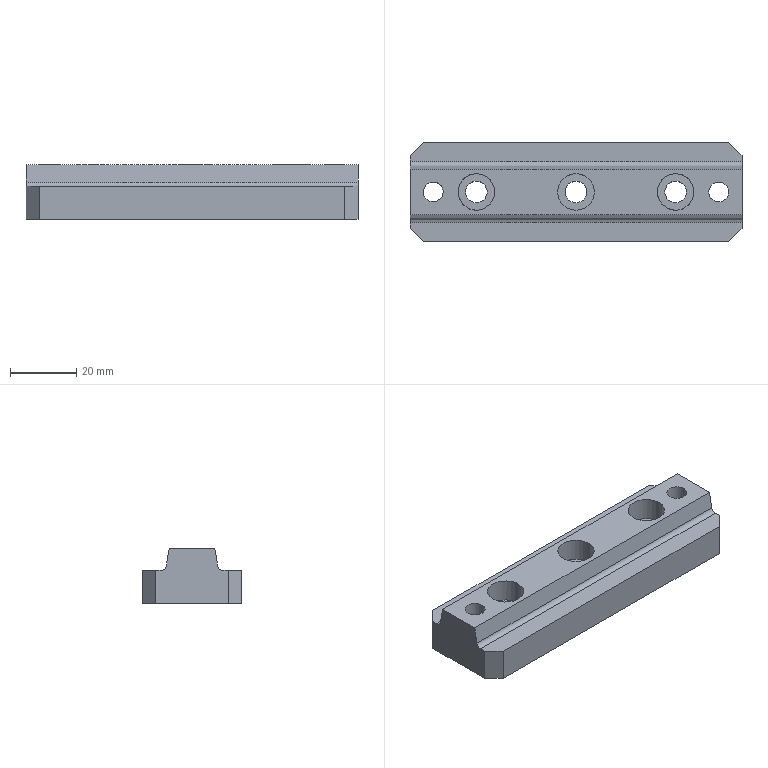Part | STEP file | 车灯-后视镜_id54_x_t | 1 solid | 27 faces | box 100 x 30 x 16.5 mm | volume 35524 mm3 | plane 17 | cylinder 10 | commonest cylinder face diameters 6.5 x3 11 x3 3 x2 6 x2
STEP:
#1=CARTESIAN_POINT('',(46.,250.,-1.5));
#2=VERTEX_POINT('',#1);
#3=CARTESIAN_POINT('',(-46.,250.,-1.5));
#4=VERTEX_POINT('',#3);
#5=CARTESIAN_POINT('',(0.,250.,-1.5));
#6=DIRECTION('',(-1.,0.,0.));
#7=VECTOR('',#6,1.);
#8=LINE('',#5,#7);
#9=EDGE_CURVE('',#2,#4,#8,.T.);
#10=ORIENTED_EDGE('',*,*,#9,.T.);
#11=CARTESIAN_POINT('',(-50.,246.,-1.5));
#12=VERTEX_POINT('',#11);
#13=CARTESIAN_POINT('',(10.75,306.75,-1.5));
#14=DIRECTION('',(0.7071,0.7071,0.));
#15=VECTOR('',#14,1.);
#16=LINE('',#13,#15);
#17=EDGE_CURVE('',#12,#4,#16,.T.);
#18=ORIENTED_EDGE('',*,*,#17,.F.);
#19=CARTESIAN_POINT('',(-50.,244.259,-1.5));
#20=VERTEX_POINT('',#19);
#21=CARTESIAN_POINT('',(-50.,317.5,-1.5));
#22=DIRECTION('',(0.,-1.,0.));
#23=VECTOR('',#22,1.);
#24=LINE('',#21,#23);
#25=EDGE_CURVE('',#12,#20,#24,.T.);
#26=ORIENTED_EDGE('',*,*,#25,.T.);
#27=CARTESIAN_POINT('',(50.,244.259,-1.5));
#28=VERTEX_POINT('',#27);
#29=CARTESIAN_POINT('',(-24.,244.259,-1.5));
#30=DIRECTION('',(-1.,0.,0.));
#31=VECTOR('',#30,1.);
#32=LINE('',#29,#31);
#33=EDGE_CURVE('',#28,#20,#32,.T.);
#34=ORIENTED_EDGE('',*,*,#33,.F.);
#35=CARTESIAN_POINT('',(50.,246.,-1.5));
#36=VERTEX_POINT('',#35);
#37=CARTESIAN_POINT('',(50.,317.5,-1.5));
#38=DIRECTION('',(0.,-1.,0.));
#39=VECTOR('',#38,1.);
#40=LINE('',#37,#39);
#41=EDGE_CURVE('',#36,#28,#40,.T.);
#42=ORIENTED_EDGE('',*,*,#41,.F.);
#43=CARTESIAN_POINT('',(-10.75,306.75,-1.5));
#44=DIRECTION('',(0.7071,-0.7071,0.));
#45=VECTOR('',#44,1.);
#46=LINE('',#43,#45);
#47=EDGE_CURVE('',#2,#36,#46,.T.);
#48=ORIENTED_EDGE('',*,*,#47,.F.);
#49=EDGE_LOOP('',(#10,#18,#26,#34,#42,#48));
#50=FACE_OUTER_BOUND('',#49,.T.);
#51=CARTESIAN_POINT('',(0.,317.5,-1.5));
#52=DIRECTION('',(0.,0.,1.));
#53=DIRECTION('',(1.,0.,0.));
#54=AXIS2_PLACEMENT_3D('',#51,#52,#53);
#55=PLANE('',#54);
#56=ADVANCED_FACE('',(#50),#55,.T.);
#57=CARTESIAN_POINT('',(50.,225.741,-1.5));
#58=VERTEX_POINT('',#57);
#59=CARTESIAN_POINT('',(50.,224.,-1.5));
#60=VERTEX_POINT('',#59);
#61=CARTESIAN_POINT('',(50.,317.5,-1.5));
#62=DIRECTION('',(0.,-1.,0.));
#63=VECTOR('',#62,1.);
#64=LINE('',#61,#63);
#65=EDGE_CURVE('',#58,#60,#64,.T.);
#66=ORIENTED_EDGE('',*,*,#65,.F.);
#67=CARTESIAN_POINT('',(-50.,225.741,-1.5));
#68=VERTEX_POINT('',#67);
#69=CARTESIAN_POINT('',(0.,225.741,-1.5));
#70=DIRECTION('',(1.,0.,0.));
#71=VECTOR('',#70,1.);
#72=LINE('',#69,#71);
#73=EDGE_CURVE('',#68,#58,#72,.T.);
#74=ORIENTED_EDGE('',*,*,#73,.F.);
#75=CARTESIAN_POINT('',(-50.,224.,-1.5));
#76=VERTEX_POINT('',#75);
#77=CARTESIAN_POINT('',(-50.,317.5,-1.5));
#78=DIRECTION('',(0.,-1.,0.));
#79=VECTOR('',#78,1.);
#80=LINE('',#77,#79);
#81=EDGE_CURVE('',#68,#76,#80,.T.);
#82=ORIENTED_EDGE('',*,*,#81,.T.);
#83=CARTESIAN_POINT('',(-46.,220.,-1.5));
#84=VERTEX_POINT('',#83);
#85=CARTESIAN_POINT('',(-71.75,245.75,-1.5));
#86=DIRECTION('',(-0.7071,0.7071,0.));
#87=VECTOR('',#86,1.);
#88=LINE('',#85,#87);
#89=EDGE_CURVE('',#84,#76,#88,.T.);
#90=ORIENTED_EDGE('',*,*,#89,.F.);
#91=CARTESIAN_POINT('',(46.,220.,-1.5));
#92=VERTEX_POINT('',#91);
#93=CARTESIAN_POINT('',(0.,220.,-1.5));
#94=DIRECTION('',(-1.,0.,0.));
#95=VECTOR('',#94,1.);
#96=LINE('',#93,#95);
#97=EDGE_CURVE('',#92,#84,#96,.T.);
#98=ORIENTED_EDGE('',*,*,#97,.F.);
#99=CARTESIAN_POINT('',(71.75,245.75,-1.5));
#100=DIRECTION('',(-0.7071,-0.7071,0.));
#101=VECTOR('',#100,1.);
#102=LINE('',#99,#101);
#103=EDGE_CURVE('',#60,#92,#102,.T.);
#104=ORIENTED_EDGE('',*,*,#103,.F.);
#105=EDGE_LOOP('',(#66,#74,#82,#90,#98,#104));
#106=FACE_OUTER_BOUND('',#105,.T.);
#107=CARTESIAN_POINT('',(0.,317.5,-1.5));
#108=DIRECTION('',(0.,0.,1.));
#109=DIRECTION('',(1.,0.,0.));
#110=AXIS2_PLACEMENT_3D('',#107,#108,#109);
#111=PLANE('',#110);
#112=ADVANCED_FACE('',(#106),#111,.T.);
#113=ORIENTED_EDGE('',*,*,#81,.F.);
#114=CARTESIAN_POINT('',(-50.,227.219,-0.2605));
#115=VERTEX_POINT('',#114);
#116=CARTESIAN_POINT('',(-50.,225.741,0.));
#117=DIRECTION('',(-1.,0.,0.));
#118=DIRECTION('',(0.,0.,-1.));
#119=AXIS2_PLACEMENT_3D('',#116,#117,#118);
#120=CIRCLE('',#119,1.5);
#121=EDGE_CURVE('',#115,#68,#120,.T.);
#122=ORIENTED_EDGE('',*,*,#121,.F.);
#123=CARTESIAN_POINT('',(-50.,228.146,5.));
#124=VERTEX_POINT('',#123);
#125=CARTESIAN_POINT('',(-50.,229.472,12.522));
#126=DIRECTION('',(0.,-0.1736,-0.9848));
#127=VECTOR('',#126,1.);
#128=LINE('',#125,#127);
#129=EDGE_CURVE('',#124,#115,#128,.T.);
#130=ORIENTED_EDGE('',*,*,#129,.F.);
#131=CARTESIAN_POINT('',(-50.,241.854,5.));
#132=VERTEX_POINT('',#131);
#133=CARTESIAN_POINT('',(-50.,317.5,5.));
#134=DIRECTION('',(0.,-1.,0.));
#135=VECTOR('',#134,1.);
#136=LINE('',#133,#135);
#137=EDGE_CURVE('',#132,#124,#136,.T.);
#138=ORIENTED_EDGE('',*,*,#137,.F.);
#139=CARTESIAN_POINT('',(-50.,242.781,-0.2605));
#140=VERTEX_POINT('',#139);
#141=CARTESIAN_POINT('',(-50.,243.,-1.5));
#142=DIRECTION('',(0.,0.1736,-0.9848));
#143=VECTOR('',#142,1.);
#144=LINE('',#141,#143);
#145=EDGE_CURVE('',#132,#140,#144,.T.);
#146=ORIENTED_EDGE('',*,*,#145,.T.);
#147=CARTESIAN_POINT('',(-50.,244.259,0.));
#148=DIRECTION('',(-1.,0.,0.));
#149=DIRECTION('',(0.,0.,-1.));
#150=AXIS2_PLACEMENT_3D('',#147,#148,#149);
#151=CIRCLE('',#150,1.5);
#152=EDGE_CURVE('',#20,#140,#151,.T.);
#153=ORIENTED_EDGE('',*,*,#152,.F.);
#154=ORIENTED_EDGE('',*,*,#25,.F.);
#155=CARTESIAN_POINT('',(-50.,246.,-11.5));
#156=VERTEX_POINT('',#155);
#157=CARTESIAN_POINT('',(-50.,246.,-3.));
#158=DIRECTION('',(0.,0.,1.));
#159=VECTOR('',#158,1.);
#160=LINE('',#157,#159);
#161=EDGE_CURVE('',#156,#12,#160,.T.);
#162=ORIENTED_EDGE('',*,*,#161,.F.);
#163=CARTESIAN_POINT('',(-50.,224.,-11.5));
#164=VERTEX_POINT('',#163);
#165=CARTESIAN_POINT('',(-50.,317.5,-11.5));
#166=DIRECTION('',(0.,1.,0.));
#167=VECTOR('',#166,1.);
#168=LINE('',#165,#167);
#169=EDGE_CURVE('',#164,#156,#168,.T.);
#170=ORIENTED_EDGE('',*,*,#169,.F.);
#171=CARTESIAN_POINT('',(-50.,224.,-3.));
#172=DIRECTION('',(0.,0.,-1.));
#173=VECTOR('',#172,1.);
#174=LINE('',#171,#173);
#175=EDGE_CURVE('',#76,#164,#174,.T.);
#176=ORIENTED_EDGE('',*,*,#175,.F.);
#177=EDGE_LOOP('',(#113,#122,#130,#138,#146,#153,#154,#162,#170,#176));
#178=FACE_OUTER_BOUND('',#177,.T.);
#179=CARTESIAN_POINT('',(-50.,317.5,-3.));
#180=DIRECTION('',(1.,0.,0.));
#181=DIRECTION('',(0.,0.,-1.));
#182=AXIS2_PLACEMENT_3D('',#179,#180,#181);
#183=PLANE('',#182);
#184=ADVANCED_FACE('',(#178),#183,.F.);
#185=ORIENTED_EDGE('',*,*,#97,.T.);
#186=CARTESIAN_POINT('',(-46.,220.,-11.5));
#187=VERTEX_POINT('',#186);
#188=CARTESIAN_POINT('',(-46.,220.,-3.5));
#189=DIRECTION('',(0.,0.,1.));
#190=VECTOR('',#189,1.);
#191=LINE('',#188,#190);
#192=EDGE_CURVE('',#187,#84,#191,.T.);
#193=ORIENTED_EDGE('',*,*,#192,.F.);
#194=CARTESIAN_POINT('',(46.,220.,-11.5));
#195=VERTEX_POINT('',#194);
#196=CARTESIAN_POINT('',(0.,220.,-11.5));
#197=DIRECTION('',(1.,0.,0.));
#198=VECTOR('',#197,1.);
#199=LINE('',#196,#198);
#200=EDGE_CURVE('',#187,#195,#199,.T.);
#201=ORIENTED_EDGE('',*,*,#200,.T.);
#202=CARTESIAN_POINT('',(46.,220.,-3.));
#203=DIRECTION('',(0.,0.,-1.));
#204=VECTOR('',#203,1.);
#205=LINE('',#202,#204);
#206=EDGE_CURVE('',#92,#195,#205,.T.);
#207=ORIENTED_EDGE('',*,*,#206,.F.);
#208=EDGE_LOOP('',(#185,#193,#201,#207));
#209=FACE_OUTER_BOUND('',#208,.T.);
#210=CARTESIAN_POINT('',(0.,220.,-3.));
#211=DIRECTION('',(0.,-1.,0.));
#212=DIRECTION('',(0.,0.,1.));
#213=AXIS2_PLACEMENT_3D('',#210,#211,#212);
#214=PLANE('',#213);
#215=ADVANCED_FACE('',(#209),#214,.T.);
#216=CARTESIAN_POINT('',(-46.,250.,-11.5));
#217=VERTEX_POINT('',#216);
#218=CARTESIAN_POINT('',(46.,250.,-11.5));
#219=VERTEX_POINT('',#218);
#220=CARTESIAN_POINT('',(0.,250.,-11.5));
#221=DIRECTION('',(1.,0.,0.));
#222=VECTOR('',#221,1.);
#223=LINE('',#220,#222);
#224=EDGE_CURVE('',#217,#219,#223,.T.);
#225=ORIENTED_EDGE('',*,*,#224,.F.);
#226=CARTESIAN_POINT('',(-46.,250.,-3.));
#227=DIRECTION('',(0.,0.,-1.));
#228=VECTOR('',#227,1.);
#229=LINE('',#226,#228);
#230=EDGE_CURVE('',#4,#217,#229,.T.);
#231=ORIENTED_EDGE('',*,*,#230,.F.);
#232=ORIENTED_EDGE('',*,*,#9,.F.);
#233=CARTESIAN_POINT('',(46.,250.,-3.5));
#234=DIRECTION('',(0.,0.,1.));
#235=VECTOR('',#234,1.);
#236=LINE('',#233,#235);
#237=EDGE_CURVE('',#219,#2,#236,.T.);
#238=ORIENTED_EDGE('',*,*,#237,.F.);
#239=EDGE_LOOP('',(#225,#231,#232,#238));
#240=FACE_OUTER_BOUND('',#239,.T.);
#241=CARTESIAN_POINT('',(0.,250.,-3.));
#242=DIRECTION('',(0.,-1.,0.));
#243=DIRECTION('',(0.,0.,1.));
#244=AXIS2_PLACEMENT_3D('',#241,#242,#243);
#245=PLANE('',#244);
#246=ADVANCED_FACE('',(#240),#245,.F.);
#247=CARTESIAN_POINT('',(50.,224.,-11.5));
#248=VERTEX_POINT('',#247);
#249=CARTESIAN_POINT('',(50.,246.,-11.5));
#250=VERTEX_POINT('',#249);
#251=CARTESIAN_POINT('',(50.,317.5,-11.5));
#252=DIRECTION('',(0.,1.,0.));
#253=VECTOR('',#252,1.);
#254=LINE('',#251,#253);
#255=EDGE_CURVE('',#248,#250,#254,.T.);
#256=ORIENTED_EDGE('',*,*,#255,.T.);
#257=CARTESIAN_POINT('',(50.,246.,-3.));
#258=DIRECTION('',(0.,0.,-1.));
#259=VECTOR('',#258,1.);
#260=LINE('',#257,#259);
#261=EDGE_CURVE('',#36,#250,#260,.T.);
#262=ORIENTED_EDGE('',*,*,#261,.F.);
#263=ORIENTED_EDGE('',*,*,#41,.T.);
#264=CARTESIAN_POINT('',(50.,242.781,-0.2605));
#265=VERTEX_POINT('',#264);
#266=CARTESIAN_POINT('',(50.,244.259,0.));
#267=DIRECTION('',(1.,0.,0.));
#268=DIRECTION('',(0.,0.,-1.));
#269=AXIS2_PLACEMENT_3D('',#266,#267,#268);
#270=CIRCLE('',#269,1.5);
#271=EDGE_CURVE('',#265,#28,#270,.T.);
#272=ORIENTED_EDGE('',*,*,#271,.F.);
#273=CARTESIAN_POINT('',(50.,241.854,5.));
#274=VERTEX_POINT('',#273);
#275=CARTESIAN_POINT('',(50.,245.503,-15.695));
#276=DIRECTION('',(0.,0.1736,-0.9848));
#277=VECTOR('',#276,1.);
#278=LINE('',#275,#277);
#279=EDGE_CURVE('',#274,#265,#278,.T.);
#280=ORIENTED_EDGE('',*,*,#279,.F.);
#281=CARTESIAN_POINT('',(50.,228.146,5.));
#282=VERTEX_POINT('',#281);
#283=CARTESIAN_POINT('',(50.,317.5,5.));
#284=DIRECTION('',(0.,-1.,0.));
#285=VECTOR('',#284,1.);
#286=LINE('',#283,#285);
#287=EDGE_CURVE('',#274,#282,#286,.T.);
#288=ORIENTED_EDGE('',*,*,#287,.T.);
#289=CARTESIAN_POINT('',(50.,227.219,-0.2605));
#290=VERTEX_POINT('',#289);
#291=CARTESIAN_POINT('',(50.,227.,-1.5));
#292=DIRECTION('',(0.,-0.1736,-0.9848));
#293=VECTOR('',#292,1.);
#294=LINE('',#291,#293);
#295=EDGE_CURVE('',#282,#290,#294,.T.);
#296=ORIENTED_EDGE('',*,*,#295,.T.);
#297=CARTESIAN_POINT('',(50.,225.741,0.));
#298=DIRECTION('',(1.,0.,0.));
#299=DIRECTION('',(0.,0.,-1.));
#300=AXIS2_PLACEMENT_3D('',#297,#298,#299);
#301=CIRCLE('',#300,1.5);
#302=EDGE_CURVE('',#58,#290,#301,.T.);
#303=ORIENTED_EDGE('',*,*,#302,.F.);
#304=ORIENTED_EDGE('',*,*,#65,.T.);
#305=CARTESIAN_POINT('',(50.,224.,-3.));
#306=DIRECTION('',(0.,0.,1.));
#307=VECTOR('',#306,1.);
#308=LINE('',#305,#307);
#309=EDGE_CURVE('',#248,#60,#308,.T.);
#310=ORIENTED_EDGE('',*,*,#309,.F.);
#311=EDGE_LOOP('',(#256,#262,#263,#272,#280,#288,#296,#303,#304,#310));
#312=FACE_OUTER_BOUND('',#311,.T.);
#313=CARTESIAN_POINT('',(50.,317.5,-3.));
#314=DIRECTION('',(1.,0.,0.));
#315=DIRECTION('',(0.,0.,-1.));
#316=AXIS2_PLACEMENT_3D('',#313,#314,#315);
#317=PLANE('',#316);
#318=ADVANCED_FACE('',(#312),#317,.T.);
#319=CARTESIAN_POINT('',(-30.,238.25,-11.5));
#320=VERTEX_POINT('',#319);
#321=CARTESIAN_POINT('',(-30.,235.,-11.5));
#322=DIRECTION('',(0.,0.,-1.));
#323=DIRECTION('',(0.,1.,0.));
#324=AXIS2_PLACEMENT_3D('',#321,#322,#323);
#325=CIRCLE('',#324,3.25);
#326=EDGE_CURVE('',#320,#320,#325,.T.);
#327=ORIENTED_EDGE('',*,*,#326,.F.);
#328=EDGE_LOOP('',(#327));
#329=FACE_BOUND('',#328,.T.);
#330=CARTESIAN_POINT('',(30.,238.25,-11.5));
#331=VERTEX_POINT('',#330);
#332=CARTESIAN_POINT('',(30.,235.,-11.5));
#333=DIRECTION('',(0.,0.,-1.));
#334=DIRECTION('',(0.,1.,0.));
#335=AXIS2_PLACEMENT_3D('',#332,#333,#334);
#336=CIRCLE('',#335,3.25);
#337=EDGE_CURVE('',#331,#331,#336,.T.);
#338=ORIENTED_EDGE('',*,*,#337,.F.);
#339=EDGE_LOOP('',(#338));
#340=FACE_BOUND('',#339,.T.);
#341=CARTESIAN_POINT('',(0.,238.25,-11.5));
#342=VERTEX_POINT('',#341);
#343=CARTESIAN_POINT('',(0.,235.,-11.5));
#344=DIRECTION('',(0.,0.,-1.));
#345=DIRECTION('',(0.,1.,0.));
#346=AXIS2_PLACEMENT_3D('',#343,#344,#345);
#347=CIRCLE('',#346,3.25);
#348=EDGE_CURVE('',#342,#342,#347,.T.);
#349=ORIENTED_EDGE('',*,*,#348,.F.);
#350=EDGE_LOOP('',(#349));
#351=FACE_BOUND('',#350,.T.);
#352=CARTESIAN_POINT('',(40.,235.,-11.5));
#353=VERTEX_POINT('',#352);
#354=CARTESIAN_POINT('',(43.,235.,-11.5));
#355=DIRECTION('',(0.,0.,-1.));
#356=DIRECTION('',(-1.,0.,0.));
#357=AXIS2_PLACEMENT_3D('',#354,#355,#356);
#358=CIRCLE('',#357,3.);
#359=EDGE_CURVE('',#353,#353,#358,.T.);
#360=ORIENTED_EDGE('',*,*,#359,.F.);
#361=EDGE_LOOP('',(#360));
#362=FACE_BOUND('',#361,.T.);
#363=CARTESIAN_POINT('',(-46.,235.,-11.5));
#364=VERTEX_POINT('',#363);
#365=CARTESIAN_POINT('',(-43.,235.,-11.5));
#366=DIRECTION('',(0.,0.,-1.));
#367=DIRECTION('',(-1.,0.,0.));
#368=AXIS2_PLACEMENT_3D('',#365,#366,#367);
#369=CIRCLE('',#368,3.);
#370=EDGE_CURVE('',#364,#364,#369,.T.);
#371=ORIENTED_EDGE('',*,*,#370,.F.);
#372=EDGE_LOOP('',(#371));
#373=FACE_BOUND('',#372,.T.);
#374=ORIENTED_EDGE('',*,*,#200,.F.);
#375=CARTESIAN_POINT('',(-71.75,245.75,-11.5));
#376=DIRECTION('',(0.7071,-0.7071,0.));
#377=VECTOR('',#376,1.);
#378=LINE('',#375,#377);
#379=EDGE_CURVE('',#164,#187,#378,.T.);
#380=ORIENTED_EDGE('',*,*,#379,.F.);
#381=ORIENTED_EDGE('',*,*,#169,.T.);
#382=CARTESIAN_POINT('',(10.75,306.75,-11.5));
#383=DIRECTION('',(-0.7071,-0.7071,0.));
#384=VECTOR('',#383,1.);
#385=LINE('',#382,#384);
#386=EDGE_CURVE('',#217,#156,#385,.T.);
#387=ORIENTED_EDGE('',*,*,#386,.F.);
#388=ORIENTED_EDGE('',*,*,#224,.T.);
#389=CARTESIAN_POINT('',(-10.75,306.75,-11.5));
#390=DIRECTION('',(-0.7071,0.7071,0.));
#391=VECTOR('',#390,1.);
#392=LINE('',#389,#391);
#393=EDGE_CURVE('',#250,#219,#392,.T.);
#394=ORIENTED_EDGE('',*,*,#393,.F.);
#395=ORIENTED_EDGE('',*,*,#255,.F.);
#396=CARTESIAN_POINT('',(71.75,245.75,-11.5));
#397=DIRECTION('',(0.7071,0.7071,0.));
#398=VECTOR('',#397,1.);
#399=LINE('',#396,#398);
#400=EDGE_CURVE('',#195,#248,#399,.T.);
#401=ORIENTED_EDGE('',*,*,#400,.F.);
#402=EDGE_LOOP('',(#374,#380,#381,#387,#388,#394,#395,#401));
#403=FACE_BOUND('',#402,.T.);
#404=CARTESIAN_POINT('',(0.,317.5,-11.5));
#405=DIRECTION('',(0.,0.,1.));
#406=DIRECTION('',(1.,0.,0.));
#407=AXIS2_PLACEMENT_3D('',#404,#405,#406);
#408=PLANE('',#407);
#409=ADVANCED_FACE('',(#329,#340,#351,#362,#373,#403),#408,.F.);
#410=ORIENTED_EDGE('',*,*,#145,.F.);
#411=CARTESIAN_POINT('',(0.,241.854,5.));
#412=DIRECTION('',(1.,0.,0.));
#413=VECTOR('',#412,1.);
#414=LINE('',#411,#413);
#415=EDGE_CURVE('',#132,#274,#414,.T.);
#416=ORIENTED_EDGE('',*,*,#415,.T.);
#417=ORIENTED_EDGE('',*,*,#279,.T.);
#418=CARTESIAN_POINT('',(24.,242.781,-0.2605));
#419=DIRECTION('',(1.,0.,0.));
#420=VECTOR('',#419,1.);
#421=LINE('',#418,#420);
#422=EDGE_CURVE('',#140,#265,#421,.T.);
#423=ORIENTED_EDGE('',*,*,#422,.F.);
#424=EDGE_LOOP('',(#410,#416,#417,#423));
#425=FACE_OUTER_BOUND('',#424,.T.);
#426=CARTESIAN_POINT('',(-24.,243.,-1.5));
#427=DIRECTION('',(0.,0.9848,0.1736));
#428=DIRECTION('',(0.,0.1736,-0.9848));
#429=AXIS2_PLACEMENT_3D('',#426,#427,#428);
#430=PLANE('',#429);
#431=ADVANCED_FACE('',(#425),#430,.T.);
#432=ORIENTED_EDGE('',*,*,#295,.F.);
#433=CARTESIAN_POINT('',(0.,228.146,5.));
#434=DIRECTION('',(1.,0.,0.));
#435=VECTOR('',#434,1.);
#436=LINE('',#433,#435);
#437=EDGE_CURVE('',#124,#282,#436,.T.);
#438=ORIENTED_EDGE('',*,*,#437,.F.);
#439=ORIENTED_EDGE('',*,*,#129,.T.);
#440=CARTESIAN_POINT('',(24.,227.219,-0.2605));
#441=DIRECTION('',(-1.,0.,0.));
#442=VECTOR('',#441,1.);
#443=LINE('',#440,#442);
#444=EDGE_CURVE('',#290,#115,#443,.T.);
#445=ORIENTED_EDGE('',*,*,#444,.F.);
#446=EDGE_LOOP('',(#432,#438,#439,#445));
#447=FACE_OUTER_BOUND('',#446,.T.);
#448=CARTESIAN_POINT('',(24.,227.,-1.5));
#449=DIRECTION('',(0.,-0.9848,0.1736));
#450=DIRECTION('',(0.,0.1736,0.9848));
#451=AXIS2_PLACEMENT_3D('',#448,#449,#450);
#452=PLANE('',#451);
#453=ADVANCED_FACE('',(#447),#452,.T.);
#454=CARTESIAN_POINT('',(-24.5,235.,5.));
#455=VERTEX_POINT('',#454);
#456=CARTESIAN_POINT('',(-30.,235.,5.));
#457=DIRECTION('',(0.,0.,1.));
#458=DIRECTION('',(1.,0.,0.));
#459=AXIS2_PLACEMENT_3D('',#456,#457,#458);
#460=CIRCLE('',#459,5.5);
#461=EDGE_CURVE('',#455,#455,#460,.T.);
#462=ORIENTED_EDGE('',*,*,#461,.F.);
#463=EDGE_LOOP('',(#462));
#464=FACE_BOUND('',#463,.T.);
#465=CARTESIAN_POINT('',(35.5,235.,5.));
#466=VERTEX_POINT('',#465);
#467=CARTESIAN_POINT('',(30.,235.,5.));
#468=DIRECTION('',(0.,0.,1.));
#469=DIRECTION('',(1.,0.,0.));
#470=AXIS2_PLACEMENT_3D('',#467,#468,#469);
#471=CIRCLE('',#470,5.5);
#472=EDGE_CURVE('',#466,#466,#471,.T.);
#473=ORIENTED_EDGE('',*,*,#472,.F.);
#474=EDGE_LOOP('',(#473));
#475=FACE_BOUND('',#474,.T.);
#476=CARTESIAN_POINT('',(0.,240.5,5.));
#477=VERTEX_POINT('',#476);
#478=CARTESIAN_POINT('',(0.,235.,5.));
#479=DIRECTION('',(0.,0.,1.));
#480=DIRECTION('',(0.,1.,0.));
#481=AXIS2_PLACEMENT_3D('',#478,#479,#480);
#482=CIRCLE('',#481,5.5);
#483=EDGE_CURVE('',#477,#477,#482,.T.);
#484=ORIENTED_EDGE('',*,*,#483,.F.);
#485=EDGE_LOOP('',(#484));
#486=FACE_BOUND('',#485,.T.);
#487=ORIENTED_EDGE('',*,*,#287,.F.);
#488=ORIENTED_EDGE('',*,*,#415,.F.);
#489=ORIENTED_EDGE('',*,*,#137,.T.);
#490=ORIENTED_EDGE('',*,*,#437,.T.);
#491=EDGE_LOOP('',(#487,#488,#489,#490));
#492=FACE_BOUND('',#491,.T.);
#493=CARTESIAN_POINT('',(-43.,232.,5.));
#494=VERTEX_POINT('',#493);
#495=CARTESIAN_POINT('',(-43.,235.,5.));
#496=DIRECTION('',(0.,0.,1.));
#497=DIRECTION('',(0.,-1.,0.));
#498=AXIS2_PLACEMENT_3D('',#495,#496,#497);
#499=CIRCLE('',#498,3.);
#500=EDGE_CURVE('',#494,#494,#499,.T.);
#501=ORIENTED_EDGE('',*,*,#500,.F.);
#502=EDGE_LOOP('',(#501));
#503=FACE_BOUND('',#502,.T.);
#504=CARTESIAN_POINT('',(43.,232.,5.));
#505=VERTEX_POINT('',#504);
#506=CARTESIAN_POINT('',(43.,235.,5.));
#507=DIRECTION('',(0.,0.,-1.));
#508=DIRECTION('',(0.,-1.,0.));
#509=AXIS2_PLACEMENT_3D('',#506,#507,#508);
#510=CIRCLE('',#509,3.);
#511=EDGE_CURVE('',#505,#505,#510,.T.);
#512=ORIENTED_EDGE('',*,*,#511,.T.);
#513=EDGE_LOOP('',(#512));
#514=FACE_BOUND('',#513,.T.);
#515=CARTESIAN_POINT('',(0.,317.5,5.));
#516=DIRECTION('',(0.,0.,1.));
#517=DIRECTION('',(1.,0.,0.));
#518=AXIS2_PLACEMENT_3D('',#515,#516,#517);
#519=PLANE('',#518);
#520=ADVANCED_FACE('',(#464,#475,#486,#492,#503,#514),#519,.T.);
#521=ORIENTED_EDGE('',*,*,#370,.T.);
#522=EDGE_LOOP('',(#521));
#523=FACE_BOUND('',#522,.T.);
#524=ORIENTED_EDGE('',*,*,#500,.T.);
#525=EDGE_LOOP('',(#524));
#526=FACE_BOUND('',#525,.T.);
#527=CARTESIAN_POINT('',(-43.,235.,-25.5));
#528=DIRECTION('',(0.,0.,-1.));
#529=DIRECTION('',(-1.,0.,0.));
#530=AXIS2_PLACEMENT_3D('',#527,#528,#529);
#531=CYLINDRICAL_SURFACE('',#530,3.);
#532=ADVANCED_FACE('',(#523,#526),#531,.F.);
#533=ORIENTED_EDGE('',*,*,#359,.T.);
#534=EDGE_LOOP('',(#533));
#535=FACE_BOUND('',#534,.T.);
#536=ORIENTED_EDGE('',*,*,#511,.F.);
#537=EDGE_LOOP('',(#536));
#538=FACE_BOUND('',#537,.T.);
#539=CARTESIAN_POINT('',(43.,235.,-25.5));
#540=DIRECTION('',(0.,0.,-1.));
#541=DIRECTION('',(-1.,0.,0.));
#542=AXIS2_PLACEMENT_3D('',#539,#540,#541);
#543=CYLINDRICAL_SURFACE('',#542,3.);
#544=ADVANCED_FACE('',(#535,#538),#543,.F.);
#545=CARTESIAN_POINT('',(0.,238.25,-2.));
#546=VERTEX_POINT('',#545);
#547=CARTESIAN_POINT('',(0.,235.,-2.));
#548=DIRECTION('',(0.,0.,1.));
#549=DIRECTION('',(0.,1.,0.));
#550=AXIS2_PLACEMENT_3D('',#547,#548,#549);
#551=CIRCLE('',#550,3.25);
#552=EDGE_CURVE('',#546,#546,#551,.T.);
#553=ORIENTED_EDGE('',*,*,#552,.T.);
#554=EDGE_LOOP('',(#553));
#555=FACE_BOUND('',#554,.T.);
#556=ORIENTED_EDGE('',*,*,#348,.T.);
#557=EDGE_LOOP('',(#556));
#558=FACE_BOUND('',#557,.T.);
#559=CARTESIAN_POINT('',(0.,235.,-25.5));
#560=DIRECTION('',(0.,0.,-1.));
#561=DIRECTION('',(-1.,0.,0.));
#562=AXIS2_PLACEMENT_3D('',#559,#560,#561);
#563=CYLINDRICAL_SURFACE('',#562,3.25);
#564=ADVANCED_FACE('',(#555,#558),#563,.F.);
#565=ORIENTED_EDGE('',*,*,#552,.F.);
#566=EDGE_LOOP('',(#565));
#567=FACE_BOUND('',#566,.T.);
#568=CARTESIAN_POINT('',(0.,229.5,-2.));
#569=VERTEX_POINT('',#568);
#570=CARTESIAN_POINT('',(0.,235.,-2.));
#571=DIRECTION('',(0.,0.,1.));
#572=DIRECTION('',(0.,-1.,0.));
#573=AXIS2_PLACEMENT_3D('',#570,#571,#572);
#574=CIRCLE('',#573,5.5);
#575=EDGE_CURVE('',#569,#569,#574,.T.);
#576=ORIENTED_EDGE('',*,*,#575,.T.);
#577=EDGE_LOOP('',(#576));
#578=FACE_BOUND('',#577,.T.);
#579=CARTESIAN_POINT('',(0.,235.,-2.));
#580=DIRECTION('',(0.,0.,-1.));
#581=DIRECTION('',(-1.,0.,0.));
#582=AXIS2_PLACEMENT_3D('',#579,#580,#581);
#583=PLANE('',#582);
#584=ADVANCED_FACE('',(#567,#578),#583,.F.);
#585=ORIENTED_EDGE('',*,*,#575,.F.);
#586=EDGE_LOOP('',(#585));
#587=FACE_BOUND('',#586,.T.);
#588=ORIENTED_EDGE('',*,*,#483,.T.);
#589=EDGE_LOOP('',(#588));
#590=FACE_BOUND('',#589,.T.);
#591=CARTESIAN_POINT('',(0.,235.,6.5));
#592=DIRECTION('',(0.,0.,-1.));
#593=DIRECTION('',(-1.,0.,0.));
#594=AXIS2_PLACEMENT_3D('',#591,#592,#593);
#595=CYLINDRICAL_SURFACE('',#594,5.5);
#596=ADVANCED_FACE('',(#587,#590),#595,.F.);
#597=ORIENTED_EDGE('',*,*,#152,.T.);
#598=ORIENTED_EDGE('',*,*,#422,.T.);
#599=ORIENTED_EDGE('',*,*,#271,.T.);
#600=ORIENTED_EDGE('',*,*,#33,.T.);
#601=EDGE_LOOP('',(#597,#598,#599,#600));
#602=FACE_OUTER_BOUND('',#601,.T.);
#603=CARTESIAN_POINT('',(-24.,244.259,0.));
#604=DIRECTION('',(-1.,0.,0.));
#605=DIRECTION('',(0.,0.,-1.));
#606=AXIS2_PLACEMENT_3D('',#603,#604,#605);
#607=CYLINDRICAL_SURFACE('',#606,1.5);
#608=ADVANCED_FACE('',(#602),#607,.F.);
#609=ORIENTED_EDGE('',*,*,#121,.T.);
#610=ORIENTED_EDGE('',*,*,#73,.T.);
#611=ORIENTED_EDGE('',*,*,#302,.T.);
#612=ORIENTED_EDGE('',*,*,#444,.T.);
#613=EDGE_LOOP('',(#609,#610,#611,#612));
#614=FACE_OUTER_BOUND('',#613,.T.);
#615=CARTESIAN_POINT('',(0.,225.741,0.));
#616=DIRECTION('',(-1.,0.,0.));
#617=DIRECTION('',(0.,0.,-1.));
#618=AXIS2_PLACEMENT_3D('',#615,#616,#617);
#619=CYLINDRICAL_SURFACE('',#618,1.5);
#620=ADVANCED_FACE('',(#614),#619,.F.);
#621=ORIENTED_EDGE('',*,*,#472,.T.);
#622=EDGE_LOOP('',(#621));
#623=FACE_BOUND('',#622,.T.);
#624=CARTESIAN_POINT('',(30.,229.5,-2.));
#625=VERTEX_POINT('',#624);
#626=CARTESIAN_POINT('',(30.,235.,-2.));
#627=DIRECTION('',(0.,0.,1.));
#628=DIRECTION('',(0.,-1.,0.));
#629=AXIS2_PLACEMENT_3D('',#626,#627,#628);
#630=CIRCLE('',#629,5.5);
#631=EDGE_CURVE('',#625,#625,#630,.T.);
#632=ORIENTED_EDGE('',*,*,#631,.F.);
#633=EDGE_LOOP('',(#632));
#634=FACE_BOUND('',#633,.T.);
#635=CARTESIAN_POINT('',(30.,235.,5.));
#636=DIRECTION('',(0.,0.,-1.));
#637=DIRECTION('',(1.,0.,0.));
#638=AXIS2_PLACEMENT_3D('',#635,#636,#637);
#639=CYLINDRICAL_SURFACE('',#638,5.5);
#640=ADVANCED_FACE('',(#623,#634),#639,.F.);
#641=CARTESIAN_POINT('',(30.,238.25,-2.));
#642=VERTEX_POINT('',#641);
#643=CARTESIAN_POINT('',(30.,235.,-2.));
#644=DIRECTION('',(0.,0.,1.));
#645=DIRECTION('',(0.,1.,0.));
#646=AXIS2_PLACEMENT_3D('',#643,#644,#645);
#647=CIRCLE('',#646,3.25);
#648=EDGE_CURVE('',#642,#642,#647,.T.);
#649=ORIENTED_EDGE('',*,*,#648,.T.);
#650=EDGE_LOOP('',(#649));
#651=FACE_BOUND('',#650,.T.);
#652=ORIENTED_EDGE('',*,*,#337,.T.);
#653=EDGE_LOOP('',(#652));
#654=FACE_BOUND('',#653,.T.);
#655=CARTESIAN_POINT('',(30.,235.,-25.5));
#656=DIRECTION('',(0.,0.,-1.));
#657=DIRECTION('',(-1.,0.,0.));
#658=AXIS2_PLACEMENT_3D('',#655,#656,#657);
#659=CYLINDRICAL_SURFACE('',#658,3.25);
#660=ADVANCED_FACE('',(#651,#654),#659,.F.);
#661=ORIENTED_EDGE('',*,*,#648,.F.);
#662=EDGE_LOOP('',(#661));
#663=FACE_BOUND('',#662,.T.);
#664=ORIENTED_EDGE('',*,*,#631,.T.);
#665=EDGE_LOOP('',(#664));
#666=FACE_BOUND('',#665,.T.);
#667=CARTESIAN_POINT('',(30.,235.,-2.));
#668=DIRECTION('',(0.,0.,-1.));
#669=DIRECTION('',(-1.,0.,0.));
#670=AXIS2_PLACEMENT_3D('',#667,#668,#669);
#671=PLANE('',#670);
#672=ADVANCED_FACE('',(#663,#666),#671,.F.);
#673=ORIENTED_EDGE('',*,*,#461,.T.);
#674=EDGE_LOOP('',(#673));
#675=FACE_BOUND('',#674,.T.);
#676=CARTESIAN_POINT('',(-30.,229.5,-2.));
#677=VERTEX_POINT('',#676);
#678=CARTESIAN_POINT('',(-30.,235.,-2.));
#679=DIRECTION('',(0.,0.,1.));
#680=DIRECTION('',(0.,-1.,0.));
#681=AXIS2_PLACEMENT_3D('',#678,#679,#680);
#682=CIRCLE('',#681,5.5);
#683=EDGE_CURVE('',#677,#677,#682,.T.);
#684=ORIENTED_EDGE('',*,*,#683,.F.);
#685=EDGE_LOOP('',(#684));
#686=FACE_BOUND('',#685,.T.);
#687=CARTESIAN_POINT('',(-30.,235.,5.));
#688=DIRECTION('',(0.,0.,-1.));
#689=DIRECTION('',(1.,0.,0.));
#690=AXIS2_PLACEMENT_3D('',#687,#688,#689);
#691=CYLINDRICAL_SURFACE('',#690,5.5);
#692=ADVANCED_FACE('',(#675,#686),#691,.F.);
#693=CARTESIAN_POINT('',(-30.,238.25,-2.));
#694=VERTEX_POINT('',#693);
#695=CARTESIAN_POINT('',(-30.,235.,-2.));
#696=DIRECTION('',(0.,0.,1.));
#697=DIRECTION('',(0.,1.,0.));
#698=AXIS2_PLACEMENT_3D('',#695,#696,#697);
#699=CIRCLE('',#698,3.25);
#700=EDGE_CURVE('',#694,#694,#699,.T.);
#701=ORIENTED_EDGE('',*,*,#700,.T.);
#702=EDGE_LOOP('',(#701));
#703=FACE_BOUND('',#702,.T.);
#704=ORIENTED_EDGE('',*,*,#326,.T.);
#705=EDGE_LOOP('',(#704));
#706=FACE_BOUND('',#705,.T.);
#707=CARTESIAN_POINT('',(-30.,235.,-25.5));
#708=DIRECTION('',(0.,0.,-1.));
#709=DIRECTION('',(-1.,0.,0.));
#710=AXIS2_PLACEMENT_3D('',#707,#708,#709);
#711=CYLINDRICAL_SURFACE('',#710,3.25);
#712=ADVANCED_FACE('',(#703,#706),#711,.F.);
#713=ORIENTED_EDGE('',*,*,#700,.F.);
#714=EDGE_LOOP('',(#713));
#715=FACE_BOUND('',#714,.T.);
#716=ORIENTED_EDGE('',*,*,#683,.T.);
#717=EDGE_LOOP('',(#716));
#718=FACE_BOUND('',#717,.T.);
#719=CARTESIAN_POINT('',(-30.,235.,-2.));
#720=DIRECTION('',(0.,0.,-1.));
#721=DIRECTION('',(-1.,0.,0.));
#722=AXIS2_PLACEMENT_3D('',#719,#720,#721);
#723=PLANE('',#722);
#724=ADVANCED_FACE('',(#715,#718),#723,.F.);
#725=ORIENTED_EDGE('',*,*,#400,.T.);
#726=ORIENTED_EDGE('',*,*,#309,.T.);
#727=ORIENTED_EDGE('',*,*,#103,.T.);
#728=ORIENTED_EDGE('',*,*,#206,.T.);
#729=EDGE_LOOP('',(#725,#726,#727,#728));
#730=FACE_OUTER_BOUND('',#729,.T.);
#731=CARTESIAN_POINT('',(50.,224.,-3.));
#732=DIRECTION('',(-0.7071,0.7071,0.));
#733=DIRECTION('',(0.7071,0.7071,0.));
#734=AXIS2_PLACEMENT_3D('',#731,#732,#733);
#735=PLANE('',#734);
#736=ADVANCED_FACE('',(#730),#735,.F.);
#737=ORIENTED_EDGE('',*,*,#47,.T.);
#738=ORIENTED_EDGE('',*,*,#261,.T.);
#739=ORIENTED_EDGE('',*,*,#393,.T.);
#740=ORIENTED_EDGE('',*,*,#237,.T.);
#741=EDGE_LOOP('',(#737,#738,#739,#740));
#742=FACE_OUTER_BOUND('',#741,.T.);
#743=CARTESIAN_POINT('',(50.,246.,-3.));
#744=DIRECTION('',(0.7071,0.7071,0.));
#745=DIRECTION('',(0.7071,-0.7071,0.));
#746=AXIS2_PLACEMENT_3D('',#743,#744,#745);
#747=PLANE('',#746);
#748=ADVANCED_FACE('',(#742),#747,.T.);
#749=ORIENTED_EDGE('',*,*,#89,.T.);
#750=ORIENTED_EDGE('',*,*,#175,.T.);
#751=ORIENTED_EDGE('',*,*,#379,.T.);
#752=ORIENTED_EDGE('',*,*,#192,.T.);
#753=EDGE_LOOP('',(#749,#750,#751,#752));
#754=FACE_OUTER_BOUND('',#753,.T.);
#755=CARTESIAN_POINT('',(-50.,224.,-3.));
#756=DIRECTION('',(-0.7071,-0.7071,0.));
#757=DIRECTION('',(-0.7071,0.7071,0.));
#758=AXIS2_PLACEMENT_3D('',#755,#756,#757);
#759=PLANE('',#758);
#760=ADVANCED_FACE('',(#754),#759,.T.);
#761=ORIENTED_EDGE('',*,*,#386,.T.);
#762=ORIENTED_EDGE('',*,*,#161,.T.);
#763=ORIENTED_EDGE('',*,*,#17,.T.);
#764=ORIENTED_EDGE('',*,*,#230,.T.);
#765=EDGE_LOOP('',(#761,#762,#763,#764));
#766=FACE_OUTER_BOUND('',#765,.T.);
#767=CARTESIAN_POINT('',(-50.,246.,-3.));
#768=DIRECTION('',(0.7071,-0.7071,0.));
#769=DIRECTION('',(-0.7071,-0.7071,0.));
#770=AXIS2_PLACEMENT_3D('',#767,#768,#769);
#771=PLANE('',#770);
#772=ADVANCED_FACE('',(#766),#771,.F.);
#773=CLOSED_SHELL('',(#56,#112,#184,#215,#246,#318,#409,#431,#453,#520,#532,#544,#564,#584,#596,#608,#620,#640,#660,#672,#692,#712,#724,#736,#748,#760,#772));
#774=MANIFOLD_SOLID_BREP('',#773);
#775=(LENGTH_UNIT()NAMED_UNIT(*)SI_UNIT(.MILLI.,.METRE.));
#776=UNCERTAINTY_MEASURE_WITH_UNIT(LENGTH_MEASURE(0.00002),#775,'','');
#777=(NAMED_UNIT(*)PLANE_ANGLE_UNIT()SI_UNIT($,.RADIAN.));
#778=PLANE_ANGLE_MEASURE_WITH_UNIT(PLANE_ANGLE_MEASURE(0.01745),#777);
#779=DIMENSIONAL_EXPONENTS(0.,0.,0.,0.,0.,0.,0.);
#780=(CONVERSION_BASED_UNIT('DEGREE',#778)NAMED_UNIT(#779)PLANE_ANGLE_UNIT());
#781=(NAMED_UNIT(*)SI_UNIT($,.STERADIAN.)SOLID_ANGLE_UNIT());
#782=(GEOMETRIC_REPRESENTATION_CONTEXT(3)GLOBAL_UNCERTAINTY_ASSIGNED_CONTEXT((#776))GLOBAL_UNIT_ASSIGNED_CONTEXT((#775,#780,#781))REPRESENTATION_CONTEXT('',''));
#783=ADVANCED_BREP_SHAPE_REPRESENTATION('',(#774),#782);